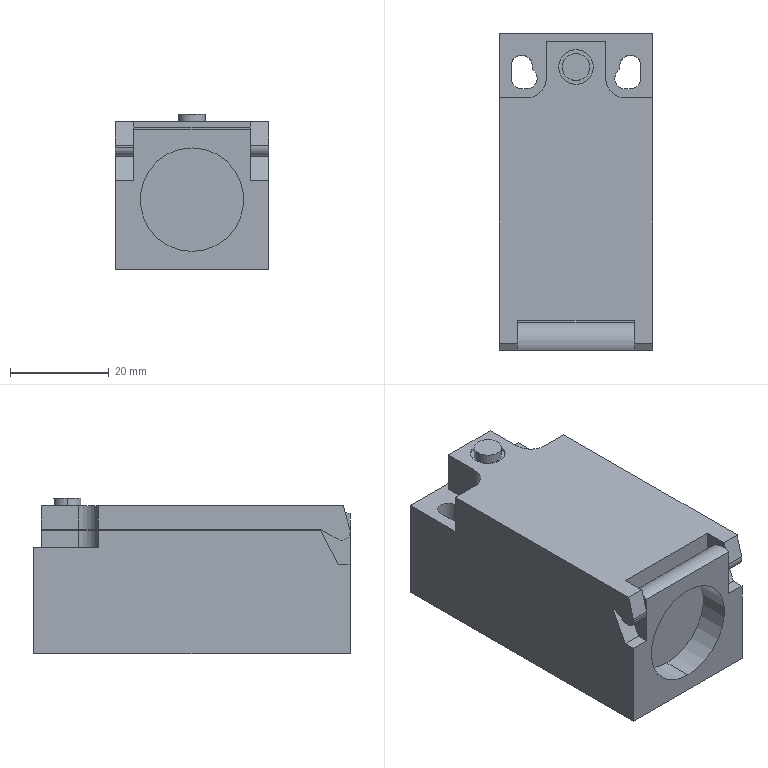Part | SolidWorks | features BaseBody 1 | 1 solid | 102 faces | box 31 x 64 x 31.5 mm | volume 53225 mm3 | plane 63 | cylinder 39 | commonest cylinder face diameters 3 x12 4.3 x7 8 x5 4 x4 3.5 x3 5.5 x2